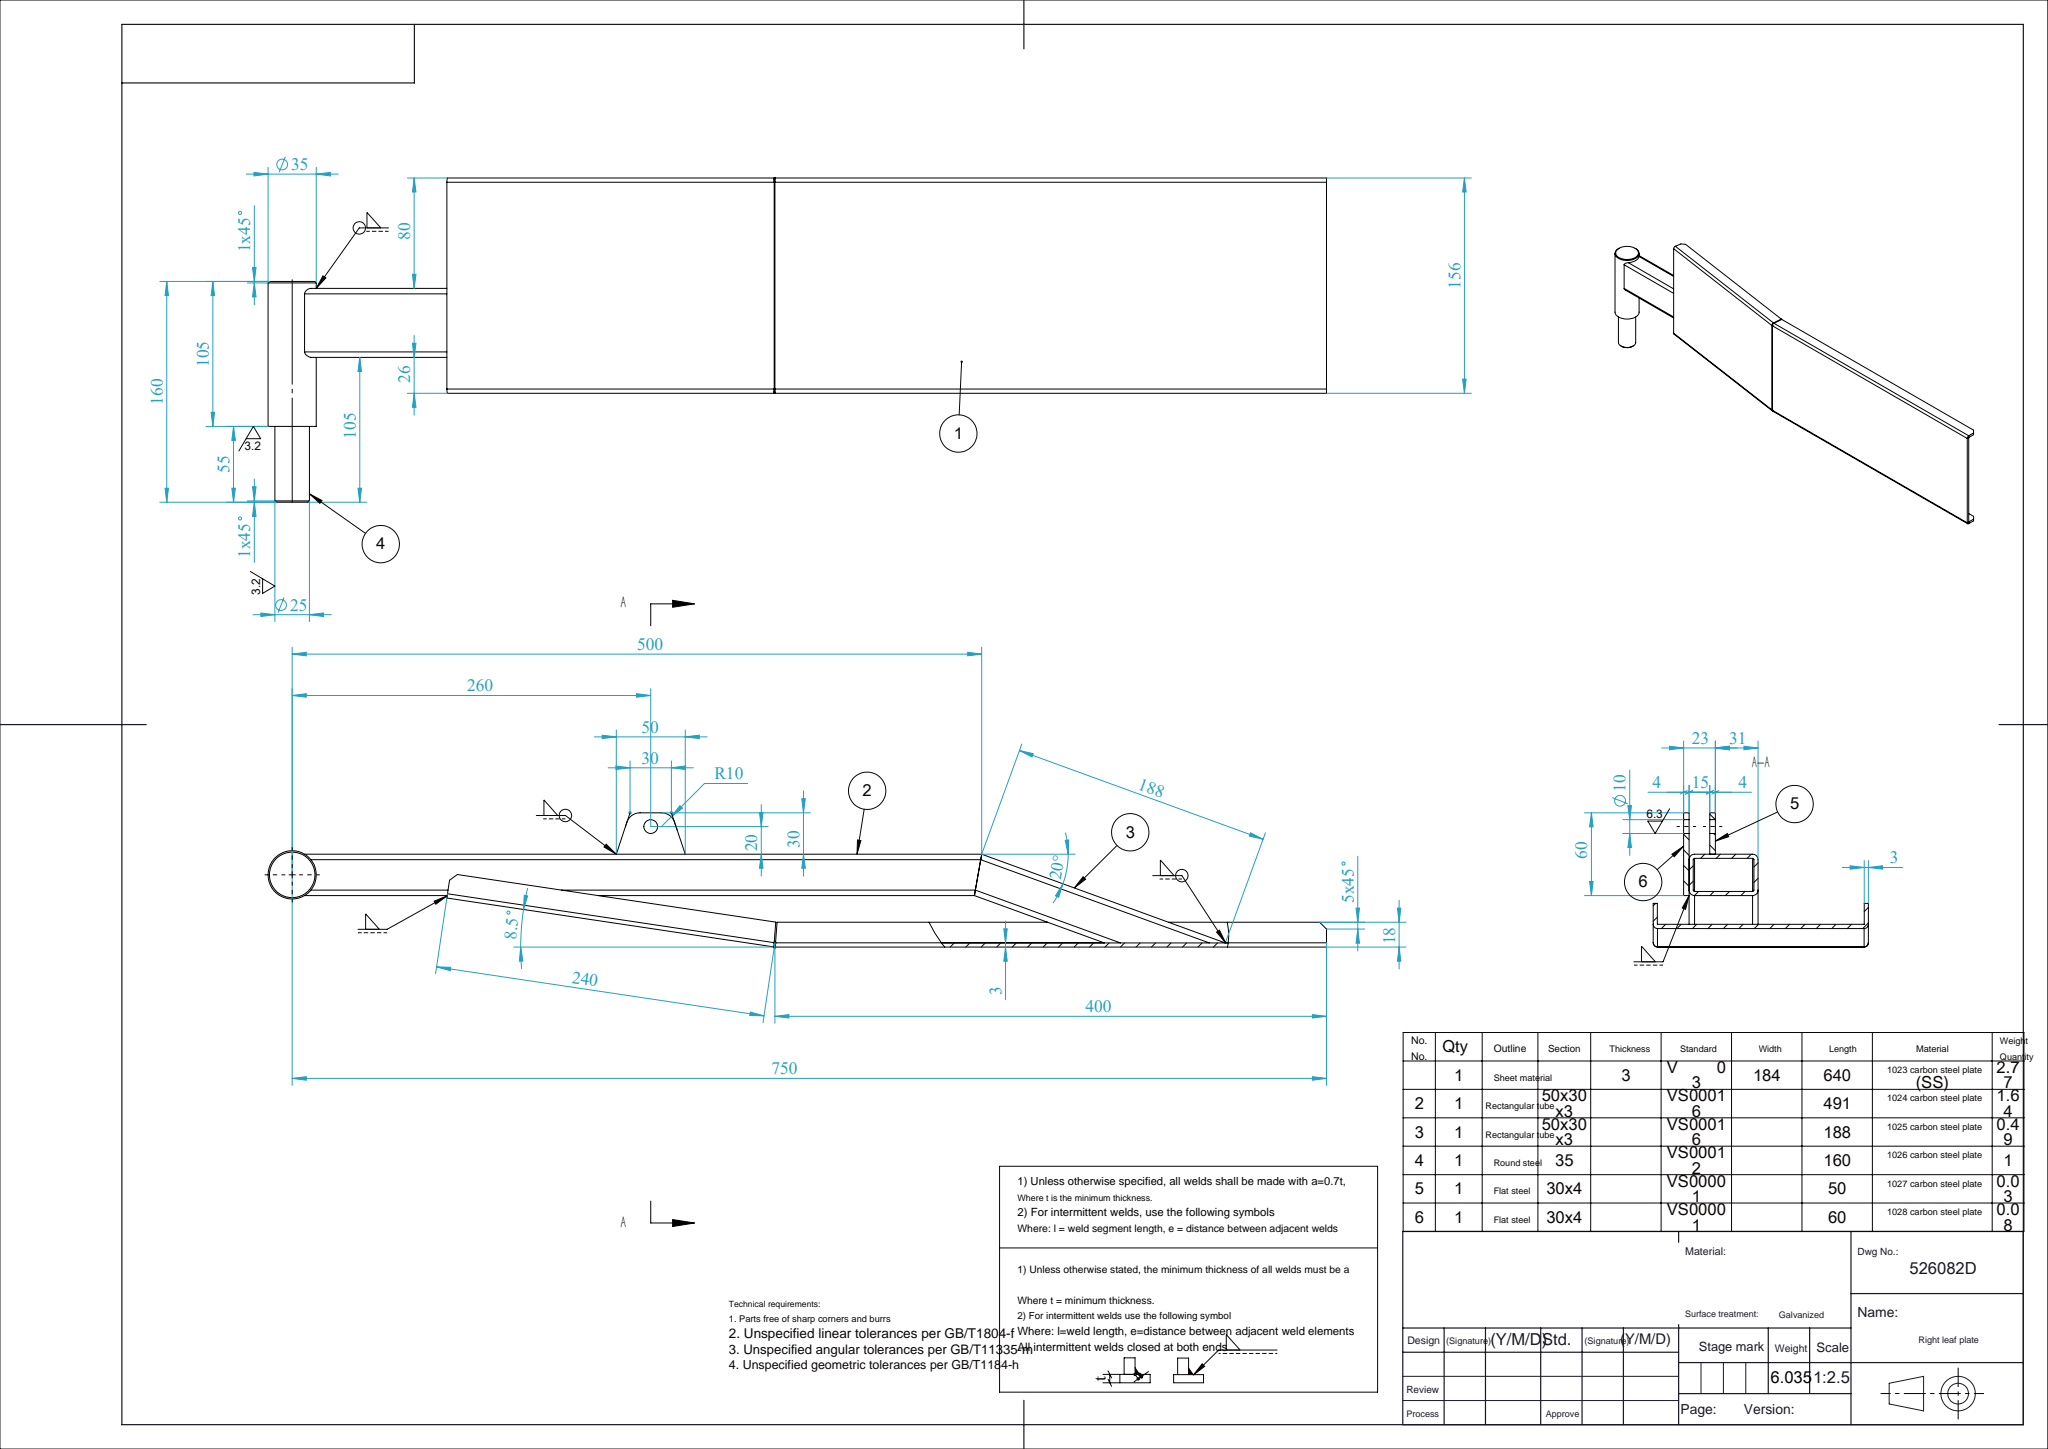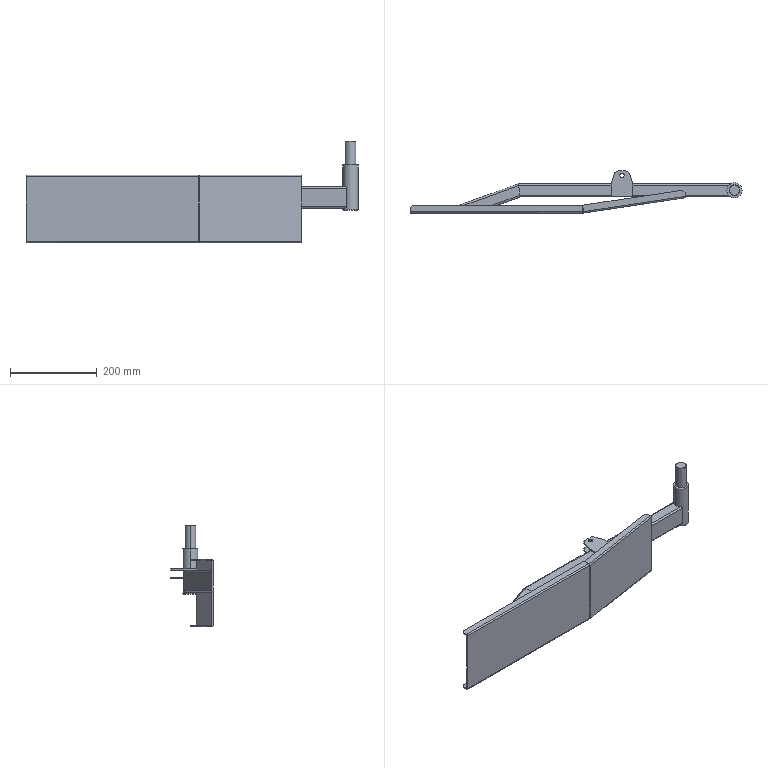Part | SolidWorks | features CompositeCurve 2 | 6 solids | 123 faces | box 767.5 x 97.3 x 235 mm | volume 768055 mm3 | plane 76 | cylinder 39 | spline 4 | cone 4 | commonest cylinder face diameters 2 x9 8 x9 0.2 x4 6.2 x4 10 x4 20 x4